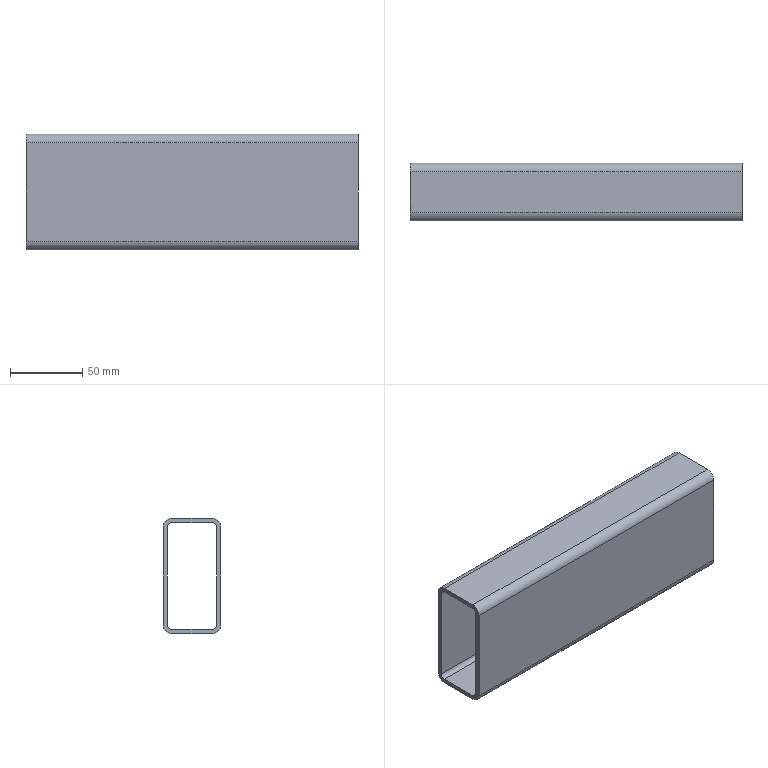Part | 1 solid | 18 faces | box 230 x 40 x 80 mm | volume 151989 mm3 | plane 10 | cylinder 8 | commonest cylinder face diameters 6 x4 12 x4
STEP:
#1=CARTESIAN_POINT('',(0.,20.,34.));
#2=VERTEX_POINT('',#1);
#3=CARTESIAN_POINT('',(0.,14.,40.));
#4=VERTEX_POINT('',#3);
#5=CARTESIAN_POINT('',(0.,14.,34.));
#6=DIRECTION('',(1.,0.,0.));
#7=DIRECTION('',(0.,0.,-1.));
#8=AXIS2_PLACEMENT_3D('',#5,#6,#7);
#9=CIRCLE('',#8,6.);
#10=EDGE_CURVE('',#2,#4,#9,.T.);
#11=ORIENTED_EDGE('',*,*,#10,.T.);
#12=CARTESIAN_POINT('',(230.,14.,40.));
#13=VERTEX_POINT('',#12);
#14=CARTESIAN_POINT('',(230.,14.,40.));
#15=DIRECTION('',(-1.,0.,0.));
#16=VECTOR('',#15,1000.);
#17=LINE('',#14,#16);
#18=EDGE_CURVE('',#13,#4,#17,.T.);
#19=ORIENTED_EDGE('',*,*,#18,.F.);
#20=CARTESIAN_POINT('',(230.,20.,34.));
#21=VERTEX_POINT('',#20);
#22=CARTESIAN_POINT('',(230.,14.,34.));
#23=DIRECTION('',(1.,0.,0.));
#24=DIRECTION('',(0.,0.,-1.));
#25=AXIS2_PLACEMENT_3D('',#22,#23,#24);
#26=CIRCLE('',#25,6.);
#27=EDGE_CURVE('',#21,#13,#26,.T.);
#28=ORIENTED_EDGE('',*,*,#27,.F.);
#29=CARTESIAN_POINT('',(230.,20.,34.));
#30=DIRECTION('',(-1.,0.,0.));
#31=VECTOR('',#30,1000.);
#32=LINE('',#29,#31);
#33=EDGE_CURVE('',#21,#2,#32,.T.);
#34=ORIENTED_EDGE('',*,*,#33,.T.);
#35=EDGE_LOOP('',(#11,#19,#28,#34));
#36=FACE_OUTER_BOUND('',#35,.T.);
#37=CARTESIAN_POINT('',(230.,14.,34.));
#38=DIRECTION('',(-1.,0.,0.));
#39=DIRECTION('',(0.,0.,1.));
#40=AXIS2_PLACEMENT_3D('',#37,#38,#39);
#41=CYLINDRICAL_SURFACE('',#40,6.);
#42=ADVANCED_FACE('',(#36),#41,.T.);
#43=CARTESIAN_POINT('',(0.,-14.,40.));
#44=VERTEX_POINT('',#43);
#45=CARTESIAN_POINT('',(0.,14.,40.));
#46=DIRECTION('',(0.,-1.,0.));
#47=VECTOR('',#46,1000.);
#48=LINE('',#45,#47);
#49=EDGE_CURVE('',#4,#44,#48,.T.);
#50=ORIENTED_EDGE('',*,*,#49,.T.);
#51=CARTESIAN_POINT('',(230.,-14.,40.));
#52=VERTEX_POINT('',#51);
#53=CARTESIAN_POINT('',(230.,-14.,40.));
#54=DIRECTION('',(-1.,0.,0.));
#55=VECTOR('',#54,1000.);
#56=LINE('',#53,#55);
#57=EDGE_CURVE('',#52,#44,#56,.T.);
#58=ORIENTED_EDGE('',*,*,#57,.F.);
#59=CARTESIAN_POINT('',(230.,14.,40.));
#60=DIRECTION('',(0.,-1.,0.));
#61=VECTOR('',#60,1000.);
#62=LINE('',#59,#61);
#63=EDGE_CURVE('',#13,#52,#62,.T.);
#64=ORIENTED_EDGE('',*,*,#63,.F.);
#65=ORIENTED_EDGE('',*,*,#18,.T.);
#66=EDGE_LOOP('',(#50,#58,#64,#65));
#67=FACE_OUTER_BOUND('',#66,.T.);
#68=CARTESIAN_POINT('',(230.,14.,40.));
#69=DIRECTION('',(0.,0.,-1.));
#70=DIRECTION('',(-1.,0.,0.));
#71=AXIS2_PLACEMENT_3D('',#68,#69,#70);
#72=PLANE('',#71);
#73=ADVANCED_FACE('',(#67),#72,.F.);
#74=CARTESIAN_POINT('',(0.,-20.,34.));
#75=VERTEX_POINT('',#74);
#76=CARTESIAN_POINT('',(0.,-14.,34.));
#77=DIRECTION('',(1.,0.,0.));
#78=DIRECTION('',(0.,0.,-1.));
#79=AXIS2_PLACEMENT_3D('',#76,#77,#78);
#80=CIRCLE('',#79,6.);
#81=EDGE_CURVE('',#44,#75,#80,.T.);
#82=ORIENTED_EDGE('',*,*,#81,.T.);
#83=CARTESIAN_POINT('',(230.,-20.,34.));
#84=VERTEX_POINT('',#83);
#85=CARTESIAN_POINT('',(230.,-20.,34.));
#86=DIRECTION('',(-1.,0.,0.));
#87=VECTOR('',#86,1000.);
#88=LINE('',#85,#87);
#89=EDGE_CURVE('',#84,#75,#88,.T.);
#90=ORIENTED_EDGE('',*,*,#89,.F.);
#91=CARTESIAN_POINT('',(230.,-14.,34.));
#92=DIRECTION('',(1.,0.,0.));
#93=DIRECTION('',(0.,0.,-1.));
#94=AXIS2_PLACEMENT_3D('',#91,#92,#93);
#95=CIRCLE('',#94,6.);
#96=EDGE_CURVE('',#52,#84,#95,.T.);
#97=ORIENTED_EDGE('',*,*,#96,.F.);
#98=ORIENTED_EDGE('',*,*,#57,.T.);
#99=EDGE_LOOP('',(#82,#90,#97,#98));
#100=FACE_OUTER_BOUND('',#99,.T.);
#101=CARTESIAN_POINT('',(230.,-14.,34.));
#102=DIRECTION('',(-1.,0.,0.));
#103=DIRECTION('',(0.,0.,1.));
#104=AXIS2_PLACEMENT_3D('',#101,#102,#103);
#105=CYLINDRICAL_SURFACE('',#104,6.);
#106=ADVANCED_FACE('',(#100),#105,.T.);
#107=CARTESIAN_POINT('',(0.,-20.,-34.));
#108=VERTEX_POINT('',#107);
#109=CARTESIAN_POINT('',(0.,-20.,-34.));
#110=DIRECTION('',(0.,0.,-1.));
#111=VECTOR('',#110,1000.);
#112=LINE('',#109,#111);
#113=EDGE_CURVE('',#75,#108,#112,.T.);
#114=ORIENTED_EDGE('',*,*,#113,.T.);
#115=CARTESIAN_POINT('',(230.,-20.,-34.));
#116=VERTEX_POINT('',#115);
#117=CARTESIAN_POINT('',(230.,-20.,-34.));
#118=DIRECTION('',(-1.,0.,0.));
#119=VECTOR('',#118,1000.);
#120=LINE('',#117,#119);
#121=EDGE_CURVE('',#116,#108,#120,.T.);
#122=ORIENTED_EDGE('',*,*,#121,.F.);
#123=CARTESIAN_POINT('',(230.,-20.,-34.));
#124=DIRECTION('',(0.,0.,-1.));
#125=VECTOR('',#124,1000.);
#126=LINE('',#123,#125);
#127=EDGE_CURVE('',#84,#116,#126,.T.);
#128=ORIENTED_EDGE('',*,*,#127,.F.);
#129=ORIENTED_EDGE('',*,*,#89,.T.);
#130=EDGE_LOOP('',(#114,#122,#128,#129));
#131=FACE_OUTER_BOUND('',#130,.T.);
#132=CARTESIAN_POINT('',(230.,-20.,-34.));
#133=DIRECTION('',(0.,1.,0.));
#134=DIRECTION('',(0.,0.,1.));
#135=AXIS2_PLACEMENT_3D('',#132,#133,#134);
#136=PLANE('',#135);
#137=ADVANCED_FACE('',(#131),#136,.F.);
#138=CARTESIAN_POINT('',(0.,-14.,-40.));
#139=VERTEX_POINT('',#138);
#140=CARTESIAN_POINT('',(0.,-14.,-34.));
#141=DIRECTION('',(1.,0.,0.));
#142=DIRECTION('',(0.,0.,-1.));
#143=AXIS2_PLACEMENT_3D('',#140,#141,#142);
#144=CIRCLE('',#143,6.);
#145=EDGE_CURVE('',#108,#139,#144,.T.);
#146=ORIENTED_EDGE('',*,*,#145,.T.);
#147=CARTESIAN_POINT('',(230.,-14.,-40.));
#148=VERTEX_POINT('',#147);
#149=CARTESIAN_POINT('',(230.,-14.,-40.));
#150=DIRECTION('',(-1.,0.,0.));
#151=VECTOR('',#150,1000.);
#152=LINE('',#149,#151);
#153=EDGE_CURVE('',#148,#139,#152,.T.);
#154=ORIENTED_EDGE('',*,*,#153,.F.);
#155=CARTESIAN_POINT('',(230.,-14.,-34.));
#156=DIRECTION('',(1.,0.,0.));
#157=DIRECTION('',(0.,0.,-1.));
#158=AXIS2_PLACEMENT_3D('',#155,#156,#157);
#159=CIRCLE('',#158,6.);
#160=EDGE_CURVE('',#116,#148,#159,.T.);
#161=ORIENTED_EDGE('',*,*,#160,.F.);
#162=ORIENTED_EDGE('',*,*,#121,.T.);
#163=EDGE_LOOP('',(#146,#154,#161,#162));
#164=FACE_OUTER_BOUND('',#163,.T.);
#165=CARTESIAN_POINT('',(230.,-14.,-34.));
#166=DIRECTION('',(-1.,0.,0.));
#167=DIRECTION('',(0.,0.,1.));
#168=AXIS2_PLACEMENT_3D('',#165,#166,#167);
#169=CYLINDRICAL_SURFACE('',#168,6.);
#170=ADVANCED_FACE('',(#164),#169,.T.);
#171=CARTESIAN_POINT('',(0.,14.,-40.));
#172=VERTEX_POINT('',#171);
#173=CARTESIAN_POINT('',(0.,-14.,-40.));
#174=DIRECTION('',(0.,1.,0.));
#175=VECTOR('',#174,1000.);
#176=LINE('',#173,#175);
#177=EDGE_CURVE('',#139,#172,#176,.T.);
#178=ORIENTED_EDGE('',*,*,#177,.T.);
#179=CARTESIAN_POINT('',(230.,14.,-40.));
#180=VERTEX_POINT('',#179);
#181=CARTESIAN_POINT('',(230.,14.,-40.));
#182=DIRECTION('',(-1.,0.,0.));
#183=VECTOR('',#182,1000.);
#184=LINE('',#181,#183);
#185=EDGE_CURVE('',#180,#172,#184,.T.);
#186=ORIENTED_EDGE('',*,*,#185,.F.);
#187=CARTESIAN_POINT('',(230.,-14.,-40.));
#188=DIRECTION('',(0.,1.,0.));
#189=VECTOR('',#188,1000.);
#190=LINE('',#187,#189);
#191=EDGE_CURVE('',#148,#180,#190,.T.);
#192=ORIENTED_EDGE('',*,*,#191,.F.);
#193=ORIENTED_EDGE('',*,*,#153,.T.);
#194=EDGE_LOOP('',(#178,#186,#192,#193));
#195=FACE_OUTER_BOUND('',#194,.T.);
#196=CARTESIAN_POINT('',(230.,-14.,-40.));
#197=DIRECTION('',(0.,0.,1.));
#198=DIRECTION('',(1.,0.,0.));
#199=AXIS2_PLACEMENT_3D('',#196,#197,#198);
#200=PLANE('',#199);
#201=ADVANCED_FACE('',(#195),#200,.F.);
#202=CARTESIAN_POINT('',(0.,20.,-34.));
#203=VERTEX_POINT('',#202);
#204=CARTESIAN_POINT('',(0.,14.,-34.));
#205=DIRECTION('',(1.,0.,0.));
#206=DIRECTION('',(0.,0.,-1.));
#207=AXIS2_PLACEMENT_3D('',#204,#205,#206);
#208=CIRCLE('',#207,6.);
#209=EDGE_CURVE('',#172,#203,#208,.T.);
#210=ORIENTED_EDGE('',*,*,#209,.T.);
#211=CARTESIAN_POINT('',(230.,20.,-34.));
#212=VERTEX_POINT('',#211);
#213=CARTESIAN_POINT('',(230.,20.,-34.));
#214=DIRECTION('',(-1.,0.,0.));
#215=VECTOR('',#214,1000.);
#216=LINE('',#213,#215);
#217=EDGE_CURVE('',#212,#203,#216,.T.);
#218=ORIENTED_EDGE('',*,*,#217,.F.);
#219=CARTESIAN_POINT('',(230.,14.,-34.));
#220=DIRECTION('',(1.,0.,0.));
#221=DIRECTION('',(0.,0.,-1.));
#222=AXIS2_PLACEMENT_3D('',#219,#220,#221);
#223=CIRCLE('',#222,6.);
#224=EDGE_CURVE('',#180,#212,#223,.T.);
#225=ORIENTED_EDGE('',*,*,#224,.F.);
#226=ORIENTED_EDGE('',*,*,#185,.T.);
#227=EDGE_LOOP('',(#210,#218,#225,#226));
#228=FACE_OUTER_BOUND('',#227,.T.);
#229=CARTESIAN_POINT('',(230.,14.,-34.));
#230=DIRECTION('',(-1.,0.,0.));
#231=DIRECTION('',(0.,0.,1.));
#232=AXIS2_PLACEMENT_3D('',#229,#230,#231);
#233=CYLINDRICAL_SURFACE('',#232,6.);
#234=ADVANCED_FACE('',(#228),#233,.T.);
#235=CARTESIAN_POINT('',(0.,-14.,37.));
#236=VERTEX_POINT('',#235);
#237=CARTESIAN_POINT('',(0.,-17.,34.));
#238=VERTEX_POINT('',#237);
#239=CARTESIAN_POINT('',(0.,-14.,34.));
#240=DIRECTION('',(1.,0.,0.));
#241=DIRECTION('',(0.,0.,-1.));
#242=AXIS2_PLACEMENT_3D('',#239,#240,#241);
#243=CIRCLE('',#242,3.);
#244=EDGE_CURVE('',#236,#238,#243,.T.);
#245=ORIENTED_EDGE('',*,*,#244,.F.);
#246=CARTESIAN_POINT('',(230.,-14.,37.));
#247=VERTEX_POINT('',#246);
#248=CARTESIAN_POINT('',(230.,-14.,37.));
#249=DIRECTION('',(-1.,0.,0.));
#250=VECTOR('',#249,1000.);
#251=LINE('',#248,#250);
#252=EDGE_CURVE('',#247,#236,#251,.T.);
#253=ORIENTED_EDGE('',*,*,#252,.F.);
#254=CARTESIAN_POINT('',(230.,-17.,34.));
#255=VERTEX_POINT('',#254);
#256=CARTESIAN_POINT('',(230.,-14.,34.));
#257=DIRECTION('',(1.,0.,0.));
#258=DIRECTION('',(0.,0.,-1.));
#259=AXIS2_PLACEMENT_3D('',#256,#257,#258);
#260=CIRCLE('',#259,3.);
#261=EDGE_CURVE('',#247,#255,#260,.T.);
#262=ORIENTED_EDGE('',*,*,#261,.T.);
#263=CARTESIAN_POINT('',(230.,-17.,34.));
#264=DIRECTION('',(-1.,0.,0.));
#265=VECTOR('',#264,1000.);
#266=LINE('',#263,#265);
#267=EDGE_CURVE('',#255,#238,#266,.T.);
#268=ORIENTED_EDGE('',*,*,#267,.T.);
#269=EDGE_LOOP('',(#245,#253,#262,#268));
#270=FACE_OUTER_BOUND('',#269,.T.);
#271=CARTESIAN_POINT('',(230.,-14.,34.));
#272=DIRECTION('',(-1.,0.,0.));
#273=DIRECTION('',(0.,0.,1.));
#274=AXIS2_PLACEMENT_3D('',#271,#272,#273);
#275=CYLINDRICAL_SURFACE('',#274,3.);
#276=ADVANCED_FACE('',(#270),#275,.F.);
#277=CARTESIAN_POINT('',(0.,14.,37.));
#278=VERTEX_POINT('',#277);
#279=CARTESIAN_POINT('',(0.,14.,37.));
#280=DIRECTION('',(0.,-1.,0.));
#281=VECTOR('',#280,1000.);
#282=LINE('',#279,#281);
#283=EDGE_CURVE('',#278,#236,#282,.T.);
#284=ORIENTED_EDGE('',*,*,#283,.F.);
#285=CARTESIAN_POINT('',(230.,14.,37.));
#286=VERTEX_POINT('',#285);
#287=CARTESIAN_POINT('',(230.,14.,37.));
#288=DIRECTION('',(-1.,0.,0.));
#289=VECTOR('',#288,1000.);
#290=LINE('',#287,#289);
#291=EDGE_CURVE('',#286,#278,#290,.T.);
#292=ORIENTED_EDGE('',*,*,#291,.F.);
#293=CARTESIAN_POINT('',(230.,14.,37.));
#294=DIRECTION('',(0.,-1.,0.));
#295=VECTOR('',#294,1000.);
#296=LINE('',#293,#295);
#297=EDGE_CURVE('',#286,#247,#296,.T.);
#298=ORIENTED_EDGE('',*,*,#297,.T.);
#299=ORIENTED_EDGE('',*,*,#252,.T.);
#300=EDGE_LOOP('',(#284,#292,#298,#299));
#301=FACE_OUTER_BOUND('',#300,.T.);
#302=CARTESIAN_POINT('',(230.,14.,37.));
#303=DIRECTION('',(0.,0.,-1.));
#304=DIRECTION('',(-1.,0.,0.));
#305=AXIS2_PLACEMENT_3D('',#302,#303,#304);
#306=PLANE('',#305);
#307=ADVANCED_FACE('',(#301),#306,.T.);
#308=CARTESIAN_POINT('',(0.,17.,34.));
#309=VERTEX_POINT('',#308);
#310=CARTESIAN_POINT('',(0.,14.,34.));
#311=DIRECTION('',(1.,0.,0.));
#312=DIRECTION('',(0.,0.,-1.));
#313=AXIS2_PLACEMENT_3D('',#310,#311,#312);
#314=CIRCLE('',#313,3.);
#315=EDGE_CURVE('',#309,#278,#314,.T.);
#316=ORIENTED_EDGE('',*,*,#315,.F.);
#317=CARTESIAN_POINT('',(230.,17.,34.));
#318=VERTEX_POINT('',#317);
#319=CARTESIAN_POINT('',(230.,17.,34.));
#320=DIRECTION('',(-1.,0.,0.));
#321=VECTOR('',#320,1000.);
#322=LINE('',#319,#321);
#323=EDGE_CURVE('',#318,#309,#322,.T.);
#324=ORIENTED_EDGE('',*,*,#323,.F.);
#325=CARTESIAN_POINT('',(230.,14.,34.));
#326=DIRECTION('',(1.,0.,0.));
#327=DIRECTION('',(0.,0.,-1.));
#328=AXIS2_PLACEMENT_3D('',#325,#326,#327);
#329=CIRCLE('',#328,3.);
#330=EDGE_CURVE('',#318,#286,#329,.T.);
#331=ORIENTED_EDGE('',*,*,#330,.T.);
#332=ORIENTED_EDGE('',*,*,#291,.T.);
#333=EDGE_LOOP('',(#316,#324,#331,#332));
#334=FACE_OUTER_BOUND('',#333,.T.);
#335=CARTESIAN_POINT('',(230.,14.,34.));
#336=DIRECTION('',(-1.,0.,0.));
#337=DIRECTION('',(0.,0.,1.));
#338=AXIS2_PLACEMENT_3D('',#335,#336,#337);
#339=CYLINDRICAL_SURFACE('',#338,3.);
#340=ADVANCED_FACE('',(#334),#339,.F.);
#341=CARTESIAN_POINT('',(0.,17.,-34.));
#342=VERTEX_POINT('',#341);
#343=CARTESIAN_POINT('',(0.,17.,34.));
#344=DIRECTION('',(0.,0.,1.));
#345=VECTOR('',#344,1000.);
#346=LINE('',#343,#345);
#347=EDGE_CURVE('',#342,#309,#346,.T.);
#348=ORIENTED_EDGE('',*,*,#347,.F.);
#349=CARTESIAN_POINT('',(230.,17.,-34.));
#350=VERTEX_POINT('',#349);
#351=CARTESIAN_POINT('',(230.,17.,-34.));
#352=DIRECTION('',(-1.,0.,0.));
#353=VECTOR('',#352,1000.);
#354=LINE('',#351,#353);
#355=EDGE_CURVE('',#350,#342,#354,.T.);
#356=ORIENTED_EDGE('',*,*,#355,.F.);
#357=CARTESIAN_POINT('',(230.,17.,34.));
#358=DIRECTION('',(0.,0.,1.));
#359=VECTOR('',#358,1000.);
#360=LINE('',#357,#359);
#361=EDGE_CURVE('',#350,#318,#360,.T.);
#362=ORIENTED_EDGE('',*,*,#361,.T.);
#363=ORIENTED_EDGE('',*,*,#323,.T.);
#364=EDGE_LOOP('',(#348,#356,#362,#363));
#365=FACE_OUTER_BOUND('',#364,.T.);
#366=CARTESIAN_POINT('',(230.,17.,34.));
#367=DIRECTION('',(0.,-1.,0.));
#368=DIRECTION('',(0.,0.,-1.));
#369=AXIS2_PLACEMENT_3D('',#366,#367,#368);
#370=PLANE('',#369);
#371=ADVANCED_FACE('',(#365),#370,.T.);
#372=CARTESIAN_POINT('',(0.,14.,-37.));
#373=VERTEX_POINT('',#372);
#374=CARTESIAN_POINT('',(0.,14.,-34.));
#375=DIRECTION('',(1.,0.,0.));
#376=DIRECTION('',(0.,0.,-1.));
#377=AXIS2_PLACEMENT_3D('',#374,#375,#376);
#378=CIRCLE('',#377,3.);
#379=EDGE_CURVE('',#373,#342,#378,.T.);
#380=ORIENTED_EDGE('',*,*,#379,.F.);
#381=CARTESIAN_POINT('',(230.,14.,-37.));
#382=VERTEX_POINT('',#381);
#383=CARTESIAN_POINT('',(230.,14.,-37.));
#384=DIRECTION('',(-1.,0.,0.));
#385=VECTOR('',#384,1000.);
#386=LINE('',#383,#385);
#387=EDGE_CURVE('',#382,#373,#386,.T.);
#388=ORIENTED_EDGE('',*,*,#387,.F.);
#389=CARTESIAN_POINT('',(230.,14.,-34.));
#390=DIRECTION('',(1.,0.,0.));
#391=DIRECTION('',(0.,0.,-1.));
#392=AXIS2_PLACEMENT_3D('',#389,#390,#391);
#393=CIRCLE('',#392,3.);
#394=EDGE_CURVE('',#382,#350,#393,.T.);
#395=ORIENTED_EDGE('',*,*,#394,.T.);
#396=ORIENTED_EDGE('',*,*,#355,.T.);
#397=EDGE_LOOP('',(#380,#388,#395,#396));
#398=FACE_OUTER_BOUND('',#397,.T.);
#399=CARTESIAN_POINT('',(230.,14.,-34.));
#400=DIRECTION('',(-1.,0.,0.));
#401=DIRECTION('',(0.,0.,1.));
#402=AXIS2_PLACEMENT_3D('',#399,#400,#401);
#403=CYLINDRICAL_SURFACE('',#402,3.);
#404=ADVANCED_FACE('',(#398),#403,.F.);
#405=CARTESIAN_POINT('',(0.,-14.,-37.));
#406=VERTEX_POINT('',#405);
#407=CARTESIAN_POINT('',(0.,-14.,-37.));
#408=DIRECTION('',(0.,1.,0.));
#409=VECTOR('',#408,1000.);
#410=LINE('',#407,#409);
#411=EDGE_CURVE('',#406,#373,#410,.T.);
#412=ORIENTED_EDGE('',*,*,#411,.F.);
#413=CARTESIAN_POINT('',(230.,-14.,-37.));
#414=VERTEX_POINT('',#413);
#415=CARTESIAN_POINT('',(230.,-14.,-37.));
#416=DIRECTION('',(-1.,0.,0.));
#417=VECTOR('',#416,1000.);
#418=LINE('',#415,#417);
#419=EDGE_CURVE('',#414,#406,#418,.T.);
#420=ORIENTED_EDGE('',*,*,#419,.F.);
#421=CARTESIAN_POINT('',(230.,-14.,-37.));
#422=DIRECTION('',(0.,1.,0.));
#423=VECTOR('',#422,1000.);
#424=LINE('',#421,#423);
#425=EDGE_CURVE('',#414,#382,#424,.T.);
#426=ORIENTED_EDGE('',*,*,#425,.T.);
#427=ORIENTED_EDGE('',*,*,#387,.T.);
#428=EDGE_LOOP('',(#412,#420,#426,#427));
#429=FACE_OUTER_BOUND('',#428,.T.);
#430=CARTESIAN_POINT('',(230.,-14.,-37.));
#431=DIRECTION('',(0.,0.,1.));
#432=DIRECTION('',(1.,0.,0.));
#433=AXIS2_PLACEMENT_3D('',#430,#431,#432);
#434=PLANE('',#433);
#435=ADVANCED_FACE('',(#429),#434,.T.);
#436=CARTESIAN_POINT('',(0.,-17.,-34.));
#437=VERTEX_POINT('',#436);
#438=CARTESIAN_POINT('',(0.,-14.,-34.));
#439=DIRECTION('',(1.,0.,0.));
#440=DIRECTION('',(0.,0.,-1.));
#441=AXIS2_PLACEMENT_3D('',#438,#439,#440);
#442=CIRCLE('',#441,3.);
#443=EDGE_CURVE('',#437,#406,#442,.T.);
#444=ORIENTED_EDGE('',*,*,#443,.F.);
#445=CARTESIAN_POINT('',(230.,-17.,-34.));
#446=VERTEX_POINT('',#445);
#447=CARTESIAN_POINT('',(230.,-17.,-34.));
#448=DIRECTION('',(-1.,0.,0.));
#449=VECTOR('',#448,1000.);
#450=LINE('',#447,#449);
#451=EDGE_CURVE('',#446,#437,#450,.T.);
#452=ORIENTED_EDGE('',*,*,#451,.F.);
#453=CARTESIAN_POINT('',(230.,-14.,-34.));
#454=DIRECTION('',(1.,0.,0.));
#455=DIRECTION('',(0.,0.,-1.));
#456=AXIS2_PLACEMENT_3D('',#453,#454,#455);
#457=CIRCLE('',#456,3.);
#458=EDGE_CURVE('',#446,#414,#457,.T.);
#459=ORIENTED_EDGE('',*,*,#458,.T.);
#460=ORIENTED_EDGE('',*,*,#419,.T.);
#461=EDGE_LOOP('',(#444,#452,#459,#460));
#462=FACE_OUTER_BOUND('',#461,.T.);
#463=CARTESIAN_POINT('',(230.,-14.,-34.));
#464=DIRECTION('',(-1.,0.,0.));
#465=DIRECTION('',(0.,0.,1.));
#466=AXIS2_PLACEMENT_3D('',#463,#464,#465);
#467=CYLINDRICAL_SURFACE('',#466,3.);
#468=ADVANCED_FACE('',(#462),#467,.F.);
#469=CARTESIAN_POINT('',(0.,-17.,-34.));
#470=DIRECTION('',(0.,0.,-1.));
#471=VECTOR('',#470,1000.);
#472=LINE('',#469,#471);
#473=EDGE_CURVE('',#238,#437,#472,.T.);
#474=ORIENTED_EDGE('',*,*,#473,.F.);
#475=ORIENTED_EDGE('',*,*,#267,.F.);
#476=CARTESIAN_POINT('',(230.,-17.,-34.));
#477=DIRECTION('',(0.,0.,-1.));
#478=VECTOR('',#477,1000.);
#479=LINE('',#476,#478);
#480=EDGE_CURVE('',#255,#446,#479,.T.);
#481=ORIENTED_EDGE('',*,*,#480,.T.);
#482=ORIENTED_EDGE('',*,*,#451,.T.);
#483=EDGE_LOOP('',(#474,#475,#481,#482));
#484=FACE_OUTER_BOUND('',#483,.T.);
#485=CARTESIAN_POINT('',(230.,-17.,-34.));
#486=DIRECTION('',(0.,1.,0.));
#487=DIRECTION('',(0.,0.,1.));
#488=AXIS2_PLACEMENT_3D('',#485,#486,#487);
#489=PLANE('',#488);
#490=ADVANCED_FACE('',(#484),#489,.T.);
#491=CARTESIAN_POINT('',(0.,20.,34.));
#492=DIRECTION('',(0.,0.,1.));
#493=VECTOR('',#492,1000.);
#494=LINE('',#491,#493);
#495=EDGE_CURVE('',#203,#2,#494,.T.);
#496=ORIENTED_EDGE('',*,*,#495,.T.);
#497=ORIENTED_EDGE('',*,*,#33,.F.);
#498=CARTESIAN_POINT('',(230.,20.,34.));
#499=DIRECTION('',(0.,0.,1.));
#500=VECTOR('',#499,1000.);
#501=LINE('',#498,#500);
#502=EDGE_CURVE('',#212,#21,#501,.T.);
#503=ORIENTED_EDGE('',*,*,#502,.F.);
#504=ORIENTED_EDGE('',*,*,#217,.T.);
#505=EDGE_LOOP('',(#496,#497,#503,#504));
#506=FACE_OUTER_BOUND('',#505,.T.);
#507=CARTESIAN_POINT('',(230.,20.,34.));
#508=DIRECTION('',(0.,-1.,0.));
#509=DIRECTION('',(0.,0.,-1.));
#510=AXIS2_PLACEMENT_3D('',#507,#508,#509);
#511=PLANE('',#510);
#512=ADVANCED_FACE('',(#506),#511,.F.);
#513=ORIENTED_EDGE('',*,*,#261,.F.);
#514=ORIENTED_EDGE('',*,*,#297,.F.);
#515=ORIENTED_EDGE('',*,*,#330,.F.);
#516=ORIENTED_EDGE('',*,*,#361,.F.);
#517=ORIENTED_EDGE('',*,*,#394,.F.);
#518=ORIENTED_EDGE('',*,*,#425,.F.);
#519=ORIENTED_EDGE('',*,*,#458,.F.);
#520=ORIENTED_EDGE('',*,*,#480,.F.);
#521=EDGE_LOOP('',(#513,#514,#515,#516,#517,#518,#519,#520));
#522=FACE_BOUND('',#521,.T.);
#523=ORIENTED_EDGE('',*,*,#27,.T.);
#524=ORIENTED_EDGE('',*,*,#63,.T.);
#525=ORIENTED_EDGE('',*,*,#96,.T.);
#526=ORIENTED_EDGE('',*,*,#127,.T.);
#527=ORIENTED_EDGE('',*,*,#160,.T.);
#528=ORIENTED_EDGE('',*,*,#191,.T.);
#529=ORIENTED_EDGE('',*,*,#224,.T.);
#530=ORIENTED_EDGE('',*,*,#502,.T.);
#531=EDGE_LOOP('',(#523,#524,#525,#526,#527,#528,#529,#530));
#532=FACE_OUTER_BOUND('',#531,.T.);
#533=CARTESIAN_POINT('',(230.,14.,34.));
#534=DIRECTION('',(1.,0.,0.));
#535=DIRECTION('',(0.,0.,-1.));
#536=AXIS2_PLACEMENT_3D('',#533,#534,#535);
#537=PLANE('',#536);
#538=ADVANCED_FACE('',(#522,#532),#537,.T.);
#539=ORIENTED_EDGE('',*,*,#244,.T.);
#540=ORIENTED_EDGE('',*,*,#473,.T.);
#541=ORIENTED_EDGE('',*,*,#443,.T.);
#542=ORIENTED_EDGE('',*,*,#411,.T.);
#543=ORIENTED_EDGE('',*,*,#379,.T.);
#544=ORIENTED_EDGE('',*,*,#347,.T.);
#545=ORIENTED_EDGE('',*,*,#315,.T.);
#546=ORIENTED_EDGE('',*,*,#283,.T.);
#547=EDGE_LOOP('',(#539,#540,#541,#542,#543,#544,#545,#546));
#548=FACE_BOUND('',#547,.T.);
#549=ORIENTED_EDGE('',*,*,#10,.F.);
#550=ORIENTED_EDGE('',*,*,#495,.F.);
#551=ORIENTED_EDGE('',*,*,#209,.F.);
#552=ORIENTED_EDGE('',*,*,#177,.F.);
#553=ORIENTED_EDGE('',*,*,#145,.F.);
#554=ORIENTED_EDGE('',*,*,#113,.F.);
#555=ORIENTED_EDGE('',*,*,#81,.F.);
#556=ORIENTED_EDGE('',*,*,#49,.F.);
#557=EDGE_LOOP('',(#549,#550,#551,#552,#553,#554,#555,#556));
#558=FACE_OUTER_BOUND('',#557,.T.);
#559=CARTESIAN_POINT('',(0.,14.,34.));
#560=DIRECTION('',(1.,0.,0.));
#561=DIRECTION('',(0.,0.,-1.));
#562=AXIS2_PLACEMENT_3D('',#559,#560,#561);
#563=PLANE('',#562);
#564=ADVANCED_FACE('',(#548,#558),#563,.F.);
#565=CLOSED_SHELL('',(#42,#73,#106,#137,#170,#201,#234,#276,#307,#340,#371,#404,#435,#468,#490,#512,#538,#564));
#566=MANIFOLD_SOLID_BREP('',#565);
#567=CARTESIAN_POINT('',(0.,0.,0.));
#568=DIRECTION('',(0.,0.,1.));
#569=DIRECTION('',(1.,0.,0.));
#570=AXIS2_PLACEMENT_3D('',#567,#568,#569);
#571=(LENGTH_UNIT()NAMED_UNIT(*)SI_UNIT(.MILLI.,.METRE.));
#572=UNCERTAINTY_MEASURE_WITH_UNIT(LENGTH_MEASURE(0.00001),#571,'','');
#573=(NAMED_UNIT(*)PLANE_ANGLE_UNIT()SI_UNIT($,.RADIAN.));
#574=(NAMED_UNIT(*)SI_UNIT($,.STERADIAN.)SOLID_ANGLE_UNIT());
#575=(GEOMETRIC_REPRESENTATION_CONTEXT(3)GLOBAL_UNCERTAINTY_ASSIGNED_CONTEXT((#572))GLOBAL_UNIT_ASSIGNED_CONTEXT((#571,#573,#574))REPRESENTATION_CONTEXT('',''));
#576=ADVANCED_BREP_SHAPE_REPRESENTATION('',(#566,#570),#575);